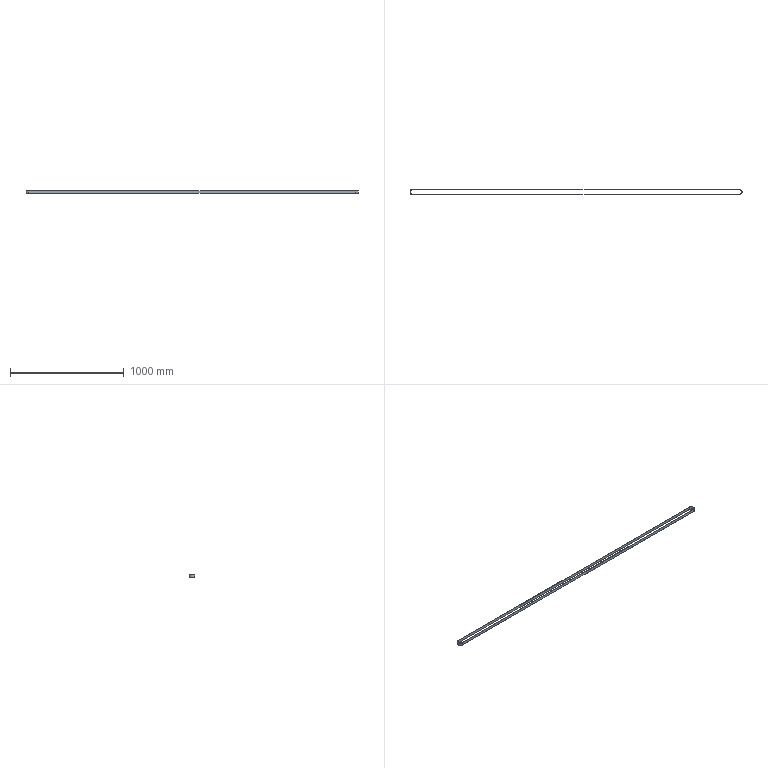Part | STEP file | Belt1-11^BPSP-03Fixture Return Conveyor Assembly_Default | 1 solid | 12 faces | box 2922 x 49 x 25 mm | volume 294683 mm3 | cylinder 6 | plane 6 | commonest cylinder face diameters 45 x3 49 x3
STEP:
#1=CARTESIAN_POINT('',(0.,0.,0.));
#2=DIRECTION('',(0.,0.,1.));
#3=DIRECTION('',(1.,0.,0.));
#4=AXIS2_PLACEMENT_3D('',#1,#2,#3);
#5=CARTESIAN_POINT('',(2873.,22.5,-25.));
#6=VERTEX_POINT('',#5);
#7=CARTESIAN_POINT('',(2873.,22.5,0.));
#8=VERTEX_POINT('',#7);
#9=CARTESIAN_POINT('',(2873.,22.5,-25.));
#10=DIRECTION('',(0.,0.,1.));
#11=VECTOR('',#10,1.);
#12=LINE('',#9,#11);
#13=CARTESIAN_POINT('',(2873.,0.000000009,-25.));
#14=DIRECTION('',(0.,0.,1.));
#15=DIRECTION('',(1.,0.,0.));
#16=AXIS2_PLACEMENT_3D('',#13,#14,#15);
#17=CYLINDRICAL_SURFACE('',#16,22.5);
#18=CARTESIAN_POINT('',(1.571,0.));
#19=DIRECTION('',(0.,1.));
#20=VECTOR('',#19,1.);
#21=LINE('',#18,#20);
#22=(GEOMETRIC_REPRESENTATION_CONTEXT(2)PARAMETRIC_REPRESENTATION_CONTEXT()REPRESENTATION_CONTEXT('',''));
#23=DEFINITIONAL_REPRESENTATION('',(#21),#22);
#24=PCURVE('',#17,#23);
#25=CARTESIAN_POINT('',(0.,22.5,-25.));
#26=DIRECTION('',(0.,1.,0.));
#27=DIRECTION('',(-1.,0.,0.));
#28=AXIS2_PLACEMENT_3D('',#25,#26,#27);
#29=PLANE('',#28);
#30=CARTESIAN_POINT('',(-2873.,0.));
#31=DIRECTION('',(0.,1.));
#32=VECTOR('',#31,1.);
#33=LINE('',#30,#32);
#34=(GEOMETRIC_REPRESENTATION_CONTEXT(2)PARAMETRIC_REPRESENTATION_CONTEXT()REPRESENTATION_CONTEXT('',''));
#35=DEFINITIONAL_REPRESENTATION('',(#33),#34);
#36=PCURVE('',#29,#35);
#37=SURFACE_CURVE('',#12,(#24,#36),.PCURVE_S1.);
#38=EDGE_CURVE('',#6,#8,#37,.T.);
#39=ORIENTED_EDGE('',*,*,#38,.T.);
#40=CARTESIAN_POINT('',(2895.5,0.000000009,0.));
#41=VERTEX_POINT('',#40);
#42=CARTESIAN_POINT('',(2873.,0.000000009,0.));
#43=DIRECTION('',(0.,0.,1.));
#44=DIRECTION('',(-1.,0.,0.));
#45=AXIS2_PLACEMENT_3D('',#42,#43,#44);
#46=CIRCLE('',#45,22.5);
#47=CARTESIAN_POINT('',(-3.142,25.));
#48=DIRECTION('',(1.,0.));
#49=VECTOR('',#48,1.);
#50=LINE('',#47,#49);
#51=(GEOMETRIC_REPRESENTATION_CONTEXT(2)PARAMETRIC_REPRESENTATION_CONTEXT()REPRESENTATION_CONTEXT('',''));
#52=DEFINITIONAL_REPRESENTATION('',(#50),#51);
#53=PCURVE('',#17,#52);
#54=CARTESIAN_POINT('',(0.,0.,0.));
#55=DIRECTION('',(0.,0.,-1.));
#56=DIRECTION('',(-1.,0.,0.));
#57=AXIS2_PLACEMENT_3D('',#54,#55,#56);
#58=PLANE('',#57);
#59=CARTESIAN_POINT('',(-2850.5,0.000000009));
#60=CARTESIAN_POINT('',(-2850.5,-38.971));
#61=CARTESIAN_POINT('',(-2884.25,-19.486));
#62=CARTESIAN_POINT('',(-2918.,0.000000009));
#63=CARTESIAN_POINT('',(-2884.25,19.486));
#64=CARTESIAN_POINT('',(-2850.5,38.971));
#65=CARTESIAN_POINT('',(-2850.5,0.000000009));
#66=(BOUNDED_CURVE()B_SPLINE_CURVE(2,(#59,#60,#61,#62,#63,#64,#65),.UNSPECIFIED.,.T.,.F.)B_SPLINE_CURVE_WITH_KNOTS((1,2,2,2,2,1),(-2.094,0.,2.094,4.189,6.283,8.378),.UNSPECIFIED.)CURVE()GEOMETRIC_REPRESENTATION_ITEM()RATIONAL_B_SPLINE_CURVE((1.,0.5,1.,0.5,1.,0.5,1.))REPRESENTATION_ITEM(''));
#67=(GEOMETRIC_REPRESENTATION_CONTEXT(2)PARAMETRIC_REPRESENTATION_CONTEXT()REPRESENTATION_CONTEXT('',''));
#68=DEFINITIONAL_REPRESENTATION('',(#66),#67);
#69=PCURVE('',#58,#68);
#70=SURFACE_CURVE('',#46,(#53,#69),.PCURVE_S1.);
#71=EDGE_CURVE('',#41,#8,#70,.T.);
#72=ORIENTED_EDGE('',*,*,#71,.F.);
#73=CARTESIAN_POINT('',(2895.5,0.000000009,-25.));
#74=VERTEX_POINT('',#73);
#75=CARTESIAN_POINT('',(2895.5,0.000000009,-25.));
#76=DIRECTION('',(0.,0.,1.));
#77=VECTOR('',#76,1.);
#78=LINE('',#75,#77);
#79=CARTESIAN_POINT('',(0.,0.));
#80=DIRECTION('',(0.,1.));
#81=VECTOR('',#80,1.);
#82=LINE('',#79,#81);
#83=(GEOMETRIC_REPRESENTATION_CONTEXT(2)PARAMETRIC_REPRESENTATION_CONTEXT()REPRESENTATION_CONTEXT('',''));
#84=DEFINITIONAL_REPRESENTATION('',(#82),#83);
#85=PCURVE('',#17,#84);
#86=CARTESIAN_POINT('',(2873.,0.000000009,-25.));
#87=DIRECTION('',(0.,0.,1.));
#88=DIRECTION('',(1.,0.,0.));
#89=AXIS2_PLACEMENT_3D('',#86,#87,#88);
#90=CYLINDRICAL_SURFACE('',#89,22.5);
#91=CARTESIAN_POINT('',(6.283,0.));
#92=DIRECTION('',(0.,1.));
#93=VECTOR('',#92,1.);
#94=LINE('',#91,#93);
#95=(GEOMETRIC_REPRESENTATION_CONTEXT(2)PARAMETRIC_REPRESENTATION_CONTEXT()REPRESENTATION_CONTEXT('',''));
#96=DEFINITIONAL_REPRESENTATION('',(#94),#95);
#97=PCURVE('',#90,#96);
#98=SURFACE_CURVE('',#78,(#85,#97),.PCURVE_S1.);
#99=EDGE_CURVE('',#74,#41,#98,.T.);
#100=ORIENTED_EDGE('',*,*,#99,.F.);
#101=CARTESIAN_POINT('',(2873.,0.000000009,-25.));
#102=DIRECTION('',(0.,0.,1.));
#103=DIRECTION('',(-1.,0.,0.));
#104=AXIS2_PLACEMENT_3D('',#101,#102,#103);
#105=CIRCLE('',#104,22.5);
#106=CARTESIAN_POINT('',(-3.142,0.));
#107=DIRECTION('',(1.,0.));
#108=VECTOR('',#107,1.);
#109=LINE('',#106,#108);
#110=(GEOMETRIC_REPRESENTATION_CONTEXT(2)PARAMETRIC_REPRESENTATION_CONTEXT()REPRESENTATION_CONTEXT('',''));
#111=DEFINITIONAL_REPRESENTATION('',(#109),#110);
#112=PCURVE('',#17,#111);
#113=CARTESIAN_POINT('',(0.,0.,-25.));
#114=DIRECTION('',(0.,0.,-1.));
#115=DIRECTION('',(-1.,0.,0.));
#116=AXIS2_PLACEMENT_3D('',#113,#114,#115);
#117=PLANE('',#116);
#118=CARTESIAN_POINT('',(-2850.5,0.000000009));
#119=CARTESIAN_POINT('',(-2850.5,-38.971));
#120=CARTESIAN_POINT('',(-2884.25,-19.486));
#121=CARTESIAN_POINT('',(-2918.,0.000000009));
#122=CARTESIAN_POINT('',(-2884.25,19.486));
#123=CARTESIAN_POINT('',(-2850.5,38.971));
#124=CARTESIAN_POINT('',(-2850.5,0.000000009));
#125=(BOUNDED_CURVE()B_SPLINE_CURVE(2,(#118,#119,#120,#121,#122,#123,#124),.UNSPECIFIED.,.T.,.F.)B_SPLINE_CURVE_WITH_KNOTS((1,2,2,2,2,1),(-2.094,0.,2.094,4.189,6.283,8.378),.UNSPECIFIED.)CURVE()GEOMETRIC_REPRESENTATION_ITEM()RATIONAL_B_SPLINE_CURVE((1.,0.5,1.,0.5,1.,0.5,1.))REPRESENTATION_ITEM(''));
#126=(GEOMETRIC_REPRESENTATION_CONTEXT(2)PARAMETRIC_REPRESENTATION_CONTEXT()REPRESENTATION_CONTEXT('',''));
#127=DEFINITIONAL_REPRESENTATION('',(#125),#126);
#128=PCURVE('',#117,#127);
#129=SURFACE_CURVE('',#105,(#112,#128),.PCURVE_S1.);
#130=EDGE_CURVE('',#74,#6,#129,.T.);
#131=ORIENTED_EDGE('',*,*,#130,.T.);
#132=EDGE_LOOP('',(#39,#72,#100,#131));
#133=FACE_BOUND('',#132,.F.);
#134=ADVANCED_FACE('',(#133),#17,.F.);
#135=CARTESIAN_POINT('',(2873.,-24.5,-25.));
#136=VERTEX_POINT('',#135);
#137=CARTESIAN_POINT('',(2897.5,0.000000009,-25.));
#138=VERTEX_POINT('',#137);
#139=CARTESIAN_POINT('',(2873.,0.000000009,-25.));
#140=DIRECTION('',(0.,0.,1.));
#141=DIRECTION('',(-1.,0.,0.));
#142=AXIS2_PLACEMENT_3D('',#139,#140,#141);
#143=CIRCLE('',#142,24.5);
#144=CARTESIAN_POINT('',(2873.,0.000000009,-25.));
#145=DIRECTION('',(0.,0.,1.));
#146=DIRECTION('',(1.,0.,0.));
#147=AXIS2_PLACEMENT_3D('',#144,#145,#146);
#148=CYLINDRICAL_SURFACE('',#147,24.5);
#149=CARTESIAN_POINT('',(3.142,0.));
#150=DIRECTION('',(1.,0.));
#151=VECTOR('',#150,1.);
#152=LINE('',#149,#151);
#153=(GEOMETRIC_REPRESENTATION_CONTEXT(2)PARAMETRIC_REPRESENTATION_CONTEXT()REPRESENTATION_CONTEXT('',''));
#154=DEFINITIONAL_REPRESENTATION('',(#152),#153);
#155=PCURVE('',#148,#154);
#156=CARTESIAN_POINT('',(-2848.5,0.000000009));
#157=CARTESIAN_POINT('',(-2848.5,-42.435));
#158=CARTESIAN_POINT('',(-2885.25,-21.218));
#159=CARTESIAN_POINT('',(-2922.,0.000000009));
#160=CARTESIAN_POINT('',(-2885.25,21.218));
#161=CARTESIAN_POINT('',(-2848.5,42.435));
#162=CARTESIAN_POINT('',(-2848.5,0.000000009));
#163=(BOUNDED_CURVE()B_SPLINE_CURVE(2,(#156,#157,#158,#159,#160,#161,#162),.UNSPECIFIED.,.T.,.F.)B_SPLINE_CURVE_WITH_KNOTS((1,2,2,2,2,1),(-2.094,0.,2.094,4.189,6.283,8.378),.UNSPECIFIED.)CURVE()GEOMETRIC_REPRESENTATION_ITEM()RATIONAL_B_SPLINE_CURVE((1.,0.5,1.,0.5,1.,0.5,1.))REPRESENTATION_ITEM(''));
#164=(GEOMETRIC_REPRESENTATION_CONTEXT(2)PARAMETRIC_REPRESENTATION_CONTEXT()REPRESENTATION_CONTEXT('',''));
#165=DEFINITIONAL_REPRESENTATION('',(#163),#164);
#166=PCURVE('',#117,#165);
#167=SURFACE_CURVE('',#143,(#155,#166),.PCURVE_S1.);
#168=EDGE_CURVE('',#136,#138,#167,.T.);
#169=ORIENTED_EDGE('',*,*,#168,.T.);
#170=CARTESIAN_POINT('',(2897.5,0.000000009,0.));
#171=VERTEX_POINT('',#170);
#172=CARTESIAN_POINT('',(2897.5,0.000000009,-25.));
#173=DIRECTION('',(0.,0.,1.));
#174=VECTOR('',#173,1.);
#175=LINE('',#172,#174);
#176=CARTESIAN_POINT('',(6.283,0.));
#177=DIRECTION('',(0.,1.));
#178=VECTOR('',#177,1.);
#179=LINE('',#176,#178);
#180=(GEOMETRIC_REPRESENTATION_CONTEXT(2)PARAMETRIC_REPRESENTATION_CONTEXT()REPRESENTATION_CONTEXT('',''));
#181=DEFINITIONAL_REPRESENTATION('',(#179),#180);
#182=PCURVE('',#148,#181);
#183=CARTESIAN_POINT('',(2873.,0.000000009,-25.));
#184=DIRECTION('',(0.,0.,1.));
#185=DIRECTION('',(1.,0.,0.));
#186=AXIS2_PLACEMENT_3D('',#183,#184,#185);
#187=CYLINDRICAL_SURFACE('',#186,24.5);
#188=CARTESIAN_POINT('',(0.,0.));
#189=DIRECTION('',(0.,1.));
#190=VECTOR('',#189,1.);
#191=LINE('',#188,#190);
#192=(GEOMETRIC_REPRESENTATION_CONTEXT(2)PARAMETRIC_REPRESENTATION_CONTEXT()REPRESENTATION_CONTEXT('',''));
#193=DEFINITIONAL_REPRESENTATION('',(#191),#192);
#194=PCURVE('',#187,#193);
#195=SURFACE_CURVE('',#175,(#182,#194),.PCURVE_S1.);
#196=EDGE_CURVE('',#138,#171,#195,.T.);
#197=ORIENTED_EDGE('',*,*,#196,.T.);
#198=CARTESIAN_POINT('',(2873.,-24.5,0.));
#199=VERTEX_POINT('',#198);
#200=CARTESIAN_POINT('',(2873.,0.000000009,0.));
#201=DIRECTION('',(0.,0.,1.));
#202=DIRECTION('',(-1.,0.,0.));
#203=AXIS2_PLACEMENT_3D('',#200,#201,#202);
#204=CIRCLE('',#203,24.5);
#205=CARTESIAN_POINT('',(3.142,25.));
#206=DIRECTION('',(1.,0.));
#207=VECTOR('',#206,1.);
#208=LINE('',#205,#207);
#209=(GEOMETRIC_REPRESENTATION_CONTEXT(2)PARAMETRIC_REPRESENTATION_CONTEXT()REPRESENTATION_CONTEXT('',''));
#210=DEFINITIONAL_REPRESENTATION('',(#208),#209);
#211=PCURVE('',#148,#210);
#212=CARTESIAN_POINT('',(-2848.5,0.000000009));
#213=CARTESIAN_POINT('',(-2848.5,-42.435));
#214=CARTESIAN_POINT('',(-2885.25,-21.218));
#215=CARTESIAN_POINT('',(-2922.,0.000000009));
#216=CARTESIAN_POINT('',(-2885.25,21.218));
#217=CARTESIAN_POINT('',(-2848.5,42.435));
#218=CARTESIAN_POINT('',(-2848.5,0.000000009));
#219=(BOUNDED_CURVE()B_SPLINE_CURVE(2,(#212,#213,#214,#215,#216,#217,#218),.UNSPECIFIED.,.T.,.F.)B_SPLINE_CURVE_WITH_KNOTS((1,2,2,2,2,1),(-2.094,0.,2.094,4.189,6.283,8.378),.UNSPECIFIED.)CURVE()GEOMETRIC_REPRESENTATION_ITEM()RATIONAL_B_SPLINE_CURVE((1.,0.5,1.,0.5,1.,0.5,1.))REPRESENTATION_ITEM(''));
#220=(GEOMETRIC_REPRESENTATION_CONTEXT(2)PARAMETRIC_REPRESENTATION_CONTEXT()REPRESENTATION_CONTEXT('',''));
#221=DEFINITIONAL_REPRESENTATION('',(#219),#220);
#222=PCURVE('',#58,#221);
#223=SURFACE_CURVE('',#204,(#211,#222),.PCURVE_S1.);
#224=EDGE_CURVE('',#199,#171,#223,.T.);
#225=ORIENTED_EDGE('',*,*,#224,.F.);
#226=CARTESIAN_POINT('',(2873.,-24.5,-25.));
#227=DIRECTION('',(0.,0.,1.));
#228=VECTOR('',#227,1.);
#229=LINE('',#226,#228);
#230=CARTESIAN_POINT('',(4.712,0.));
#231=DIRECTION('',(0.,1.));
#232=VECTOR('',#231,1.);
#233=LINE('',#230,#232);
#234=(GEOMETRIC_REPRESENTATION_CONTEXT(2)PARAMETRIC_REPRESENTATION_CONTEXT()REPRESENTATION_CONTEXT('',''));
#235=DEFINITIONAL_REPRESENTATION('',(#233),#234);
#236=PCURVE('',#148,#235);
#237=CARTESIAN_POINT('',(2873.,-24.5,-25.));
#238=DIRECTION('',(0.,-1.,0.));
#239=DIRECTION('',(1.,0.,0.));
#240=AXIS2_PLACEMENT_3D('',#237,#238,#239);
#241=PLANE('',#240);
#242=CARTESIAN_POINT('',(0.,0.));
#243=DIRECTION('',(0.,1.));
#244=VECTOR('',#243,1.);
#245=LINE('',#242,#244);
#246=(GEOMETRIC_REPRESENTATION_CONTEXT(2)PARAMETRIC_REPRESENTATION_CONTEXT()REPRESENTATION_CONTEXT('',''));
#247=DEFINITIONAL_REPRESENTATION('',(#245),#246);
#248=PCURVE('',#241,#247);
#249=SURFACE_CURVE('',#229,(#236,#248),.PCURVE_S1.);
#250=EDGE_CURVE('',#136,#199,#249,.T.);
#251=ORIENTED_EDGE('',*,*,#250,.F.);
#252=EDGE_LOOP('',(#169,#197,#225,#251));
#253=FACE_BOUND('',#252,.T.);
#254=ADVANCED_FACE('',(#253),#148,.T.);
#255=CARTESIAN_POINT('',(0.,24.5,-25.));
#256=VERTEX_POINT('',#255);
#257=CARTESIAN_POINT('',(0.,-24.5,-25.));
#258=VERTEX_POINT('',#257);
#259=CARTESIAN_POINT('',(0.,0.,-25.));
#260=DIRECTION('',(0.,0.,1.));
#261=DIRECTION('',(-1.,0.,0.));
#262=AXIS2_PLACEMENT_3D('',#259,#260,#261);
#263=CIRCLE('',#262,24.5);
#264=CARTESIAN_POINT('',(24.5,0.));
#265=CARTESIAN_POINT('',(24.5,-42.435));
#266=CARTESIAN_POINT('',(-12.25,-21.218));
#267=CARTESIAN_POINT('',(-49.,0.));
#268=CARTESIAN_POINT('',(-12.25,21.218));
#269=CARTESIAN_POINT('',(24.5,42.435));
#270=CARTESIAN_POINT('',(24.5,0.));
#271=(BOUNDED_CURVE()B_SPLINE_CURVE(2,(#264,#265,#266,#267,#268,#269,#270),.UNSPECIFIED.,.T.,.F.)B_SPLINE_CURVE_WITH_KNOTS((1,2,2,2,2,1),(-2.094,0.,2.094,4.189,6.283,8.378),.UNSPECIFIED.)CURVE()GEOMETRIC_REPRESENTATION_ITEM()RATIONAL_B_SPLINE_CURVE((1.,0.5,1.,0.5,1.,0.5,1.))REPRESENTATION_ITEM(''));
#272=(GEOMETRIC_REPRESENTATION_CONTEXT(2)PARAMETRIC_REPRESENTATION_CONTEXT()REPRESENTATION_CONTEXT('',''));
#273=DEFINITIONAL_REPRESENTATION('',(#271),#272);
#274=PCURVE('',#117,#273);
#275=CARTESIAN_POINT('',(0.,0.,-25.));
#276=DIRECTION('',(0.,0.,1.));
#277=DIRECTION('',(1.,0.,0.));
#278=AXIS2_PLACEMENT_3D('',#275,#276,#277);
#279=CYLINDRICAL_SURFACE('',#278,24.5);
#280=CARTESIAN_POINT('',(-3.142,0.));
#281=DIRECTION('',(1.,0.));
#282=VECTOR('',#281,1.);
#283=LINE('',#280,#282);
#284=(GEOMETRIC_REPRESENTATION_CONTEXT(2)PARAMETRIC_REPRESENTATION_CONTEXT()REPRESENTATION_CONTEXT('',''));
#285=DEFINITIONAL_REPRESENTATION('',(#283),#284);
#286=PCURVE('',#279,#285);
#287=SURFACE_CURVE('',#263,(#274,#286),.PCURVE_S1.);
#288=EDGE_CURVE('',#256,#258,#287,.T.);
#289=ORIENTED_EDGE('',*,*,#288,.F.);
#290=CARTESIAN_POINT('',(2873.,24.5,-25.));
#291=VERTEX_POINT('',#290);
#292=CARTESIAN_POINT('',(0.,24.5,-25.));
#293=DIRECTION('',(-1.,0.,0.));
#294=VECTOR('',#293,1.);
#295=LINE('',#292,#294);
#296=CARTESIAN_POINT('',(0.,24.5));
#297=DIRECTION('',(1.,0.));
#298=VECTOR('',#297,1.);
#299=LINE('',#296,#298);
#300=(GEOMETRIC_REPRESENTATION_CONTEXT(2)PARAMETRIC_REPRESENTATION_CONTEXT()REPRESENTATION_CONTEXT('',''));
#301=DEFINITIONAL_REPRESENTATION('',(#299),#300);
#302=PCURVE('',#117,#301);
#303=CARTESIAN_POINT('',(0.,24.5,-25.));
#304=DIRECTION('',(0.,1.,0.));
#305=DIRECTION('',(-1.,0.,0.));
#306=AXIS2_PLACEMENT_3D('',#303,#304,#305);
#307=PLANE('',#306);
#308=CARTESIAN_POINT('',(0.,0.));
#309=DIRECTION('',(1.,0.));
#310=VECTOR('',#309,1.);
#311=LINE('',#308,#310);
#312=(GEOMETRIC_REPRESENTATION_CONTEXT(2)PARAMETRIC_REPRESENTATION_CONTEXT()REPRESENTATION_CONTEXT('',''));
#313=DEFINITIONAL_REPRESENTATION('',(#311),#312);
#314=PCURVE('',#307,#313);
#315=SURFACE_CURVE('',#295,(#302,#314),.PCURVE_S1.);
#316=EDGE_CURVE('',#291,#256,#315,.T.);
#317=ORIENTED_EDGE('',*,*,#316,.F.);
#318=CARTESIAN_POINT('',(2873.,0.000000009,-25.));
#319=DIRECTION('',(0.,0.,1.));
#320=DIRECTION('',(-1.,0.,0.));
#321=AXIS2_PLACEMENT_3D('',#318,#319,#320);
#322=CIRCLE('',#321,24.5);
#323=CARTESIAN_POINT('',(-2848.5,0.000000009));
#324=CARTESIAN_POINT('',(-2848.5,-42.435));
#325=CARTESIAN_POINT('',(-2885.25,-21.218));
#326=CARTESIAN_POINT('',(-2922.,0.000000009));
#327=CARTESIAN_POINT('',(-2885.25,21.218));
#328=CARTESIAN_POINT('',(-2848.5,42.435));
#329=CARTESIAN_POINT('',(-2848.5,0.000000009));
#330=(BOUNDED_CURVE()B_SPLINE_CURVE(2,(#323,#324,#325,#326,#327,#328,#329),.UNSPECIFIED.,.T.,.F.)B_SPLINE_CURVE_WITH_KNOTS((1,2,2,2,2,1),(-2.094,0.,2.094,4.189,6.283,8.378),.UNSPECIFIED.)CURVE()GEOMETRIC_REPRESENTATION_ITEM()RATIONAL_B_SPLINE_CURVE((1.,0.5,1.,0.5,1.,0.5,1.))REPRESENTATION_ITEM(''));
#331=(GEOMETRIC_REPRESENTATION_CONTEXT(2)PARAMETRIC_REPRESENTATION_CONTEXT()REPRESENTATION_CONTEXT('',''));
#332=DEFINITIONAL_REPRESENTATION('',(#330),#331);
#333=PCURVE('',#117,#332);
#334=CARTESIAN_POINT('',(-3.142,0.));
#335=DIRECTION('',(1.,0.));
#336=VECTOR('',#335,1.);
#337=LINE('',#334,#336);
#338=(GEOMETRIC_REPRESENTATION_CONTEXT(2)PARAMETRIC_REPRESENTATION_CONTEXT()REPRESENTATION_CONTEXT('',''));
#339=DEFINITIONAL_REPRESENTATION('',(#337),#338);
#340=PCURVE('',#187,#339);
#341=SURFACE_CURVE('',#322,(#333,#340),.PCURVE_S1.);
#342=EDGE_CURVE('',#138,#291,#341,.T.);
#343=ORIENTED_EDGE('',*,*,#342,.F.);
#344=ORIENTED_EDGE('',*,*,#168,.F.);
#345=CARTESIAN_POINT('',(2873.,-24.5,-25.));
#346=DIRECTION('',(1.,0.,0.));
#347=VECTOR('',#346,1.);
#348=LINE('',#345,#347);
#349=CARTESIAN_POINT('',(-2873.,-24.5));
#350=DIRECTION('',(-1.,0.));
#351=VECTOR('',#350,1.);
#352=LINE('',#349,#351);
#353=(GEOMETRIC_REPRESENTATION_CONTEXT(2)PARAMETRIC_REPRESENTATION_CONTEXT()REPRESENTATION_CONTEXT('',''));
#354=DEFINITIONAL_REPRESENTATION('',(#352),#353);
#355=PCURVE('',#117,#354);
#356=CARTESIAN_POINT('',(0.,0.));
#357=DIRECTION('',(1.,0.));
#358=VECTOR('',#357,1.);
#359=LINE('',#356,#358);
#360=(GEOMETRIC_REPRESENTATION_CONTEXT(2)PARAMETRIC_REPRESENTATION_CONTEXT()REPRESENTATION_CONTEXT('',''));
#361=DEFINITIONAL_REPRESENTATION('',(#359),#360);
#362=PCURVE('',#241,#361);
#363=SURFACE_CURVE('',#348,(#355,#362),.PCURVE_S1.);
#364=EDGE_CURVE('',#258,#136,#363,.T.);
#365=ORIENTED_EDGE('',*,*,#364,.F.);
#366=EDGE_LOOP('',(#289,#317,#343,#344,#365));
#367=FACE_BOUND('',#366,.T.);
#368=CARTESIAN_POINT('',(0.,22.5,-25.));
#369=VERTEX_POINT('',#368);
#370=CARTESIAN_POINT('',(0.,22.5,-25.));
#371=DIRECTION('',(-1.,0.,0.));
#372=VECTOR('',#371,1.);
#373=LINE('',#370,#372);
#374=CARTESIAN_POINT('',(0.,22.5));
#375=DIRECTION('',(1.,0.));
#376=VECTOR('',#375,1.);
#377=LINE('',#374,#376);
#378=(GEOMETRIC_REPRESENTATION_CONTEXT(2)PARAMETRIC_REPRESENTATION_CONTEXT()REPRESENTATION_CONTEXT('',''));
#379=DEFINITIONAL_REPRESENTATION('',(#377),#378);
#380=PCURVE('',#117,#379);
#381=CARTESIAN_POINT('',(0.,0.));
#382=DIRECTION('',(1.,0.));
#383=VECTOR('',#382,1.);
#384=LINE('',#381,#383);
#385=(GEOMETRIC_REPRESENTATION_CONTEXT(2)PARAMETRIC_REPRESENTATION_CONTEXT()REPRESENTATION_CONTEXT('',''));
#386=DEFINITIONAL_REPRESENTATION('',(#384),#385);
#387=PCURVE('',#29,#386);
#388=SURFACE_CURVE('',#373,(#380,#387),.PCURVE_S1.);
#389=EDGE_CURVE('',#6,#369,#388,.T.);
#390=ORIENTED_EDGE('',*,*,#389,.T.);
#391=CARTESIAN_POINT('',(0.,-22.5,-25.));
#392=VERTEX_POINT('',#391);
#393=CARTESIAN_POINT('',(0.,0.,-25.));
#394=DIRECTION('',(0.,0.,1.));
#395=DIRECTION('',(-1.,0.,0.));
#396=AXIS2_PLACEMENT_3D('',#393,#394,#395);
#397=CIRCLE('',#396,22.5);
#398=CARTESIAN_POINT('',(22.5,0.));
#399=CARTESIAN_POINT('',(22.5,-38.971));
#400=CARTESIAN_POINT('',(-11.25,-19.486));
#401=CARTESIAN_POINT('',(-45.,0.));
#402=CARTESIAN_POINT('',(-11.25,19.486));
#403=CARTESIAN_POINT('',(22.5,38.971));
#404=CARTESIAN_POINT('',(22.5,0.));
#405=(BOUNDED_CURVE()B_SPLINE_CURVE(2,(#398,#399,#400,#401,#402,#403,#404),.UNSPECIFIED.,.T.,.F.)B_SPLINE_CURVE_WITH_KNOTS((1,2,2,2,2,1),(-2.094,0.,2.094,4.189,6.283,8.378),.UNSPECIFIED.)CURVE()GEOMETRIC_REPRESENTATION_ITEM()RATIONAL_B_SPLINE_CURVE((1.,0.5,1.,0.5,1.,0.5,1.))REPRESENTATION_ITEM(''));
#406=(GEOMETRIC_REPRESENTATION_CONTEXT(2)PARAMETRIC_REPRESENTATION_CONTEXT()REPRESENTATION_CONTEXT('',''));
#407=DEFINITIONAL_REPRESENTATION('',(#405),#406);
#408=PCURVE('',#117,#407);
#409=CARTESIAN_POINT('',(0.,0.,-25.));
#410=DIRECTION('',(0.,0.,1.));
#411=DIRECTION('',(1.,0.,0.));
#412=AXIS2_PLACEMENT_3D('',#409,#410,#411);
#413=CYLINDRICAL_SURFACE('',#412,22.5);
#414=CARTESIAN_POINT('',(-3.142,0.));
#415=DIRECTION('',(1.,0.));
#416=VECTOR('',#415,1.);
#417=LINE('',#414,#416);
#418=(GEOMETRIC_REPRESENTATION_CONTEXT(2)PARAMETRIC_REPRESENTATION_CONTEXT()REPRESENTATION_CONTEXT('',''));
#419=DEFINITIONAL_REPRESENTATION('',(#417),#418);
#420=PCURVE('',#413,#419);
#421=SURFACE_CURVE('',#397,(#408,#420),.PCURVE_S1.);
#422=EDGE_CURVE('',#369,#392,#421,.T.);
#423=ORIENTED_EDGE('',*,*,#422,.T.);
#424=CARTESIAN_POINT('',(2873.,-22.5,-25.));
#425=VERTEX_POINT('',#424);
#426=CARTESIAN_POINT('',(2873.,-22.5,-25.));
#427=DIRECTION('',(1.,0.,0.));
#428=VECTOR('',#427,1.);
#429=LINE('',#426,#428);
#430=CARTESIAN_POINT('',(-2873.,-22.5));
#431=DIRECTION('',(-1.,0.));
#432=VECTOR('',#431,1.);
#433=LINE('',#430,#432);
#434=(GEOMETRIC_REPRESENTATION_CONTEXT(2)PARAMETRIC_REPRESENTATION_CONTEXT()REPRESENTATION_CONTEXT('',''));
#435=DEFINITIONAL_REPRESENTATION('',(#433),#434);
#436=PCURVE('',#117,#435);
#437=CARTESIAN_POINT('',(2873.,-22.5,-25.));
#438=DIRECTION('',(0.,-1.,0.));
#439=DIRECTION('',(1.,0.,0.));
#440=AXIS2_PLACEMENT_3D('',#437,#438,#439);
#441=PLANE('',#440);
#442=CARTESIAN_POINT('',(0.,0.));
#443=DIRECTION('',(1.,0.));
#444=VECTOR('',#443,1.);
#445=LINE('',#442,#444);
#446=(GEOMETRIC_REPRESENTATION_CONTEXT(2)PARAMETRIC_REPRESENTATION_CONTEXT()REPRESENTATION_CONTEXT('',''));
#447=DEFINITIONAL_REPRESENTATION('',(#445),#446);
#448=PCURVE('',#441,#447);
#449=SURFACE_CURVE('',#429,(#436,#448),.PCURVE_S1.);
#450=EDGE_CURVE('',#392,#425,#449,.T.);
#451=ORIENTED_EDGE('',*,*,#450,.T.);
#452=CARTESIAN_POINT('',(2873.,0.000000009,-25.));
#453=DIRECTION('',(0.,0.,1.));
#454=DIRECTION('',(-1.,0.,0.));
#455=AXIS2_PLACEMENT_3D('',#452,#453,#454);
#456=CIRCLE('',#455,22.5);
#457=CARTESIAN_POINT('',(-2850.5,0.000000009));
#458=CARTESIAN_POINT('',(-2850.5,-38.971));
#459=CARTESIAN_POINT('',(-2884.25,-19.486));
#460=CARTESIAN_POINT('',(-2918.,0.000000009));
#461=CARTESIAN_POINT('',(-2884.25,19.486));
#462=CARTESIAN_POINT('',(-2850.5,38.971));
#463=CARTESIAN_POINT('',(-2850.5,0.000000009));
#464=(BOUNDED_CURVE()B_SPLINE_CURVE(2,(#457,#458,#459,#460,#461,#462,#463),.UNSPECIFIED.,.T.,.F.)B_SPLINE_CURVE_WITH_KNOTS((1,2,2,2,2,1),(-2.094,0.,2.094,4.189,6.283,8.378),.UNSPECIFIED.)CURVE()GEOMETRIC_REPRESENTATION_ITEM()RATIONAL_B_SPLINE_CURVE((1.,0.5,1.,0.5,1.,0.5,1.))REPRESENTATION_ITEM(''));
#465=(GEOMETRIC_REPRESENTATION_CONTEXT(2)PARAMETRIC_REPRESENTATION_CONTEXT()REPRESENTATION_CONTEXT('',''));
#466=DEFINITIONAL_REPRESENTATION('',(#464),#465);
#467=PCURVE('',#117,#466);
#468=CARTESIAN_POINT('',(3.142,0.));
#469=DIRECTION('',(1.,0.));
#470=VECTOR('',#469,1.);
#471=LINE('',#468,#470);
#472=(GEOMETRIC_REPRESENTATION_CONTEXT(2)PARAMETRIC_REPRESENTATION_CONTEXT()REPRESENTATION_CONTEXT('',''));
#473=DEFINITIONAL_REPRESENTATION('',(#471),#472);
#474=PCURVE('',#90,#473);
#475=SURFACE_CURVE('',#456,(#467,#474),.PCURVE_S1.);
#476=EDGE_CURVE('',#425,#74,#475,.T.);
#477=ORIENTED_EDGE('',*,*,#476,.T.);
#478=ORIENTED_EDGE('',*,*,#130,.T.);
#479=EDGE_LOOP('',(#390,#423,#451,#477,#478));
#480=FACE_BOUND('',#479,.T.);
#481=ADVANCED_FACE('',(#367,#480),#117,.T.);
#482=CARTESIAN_POINT('',(0.,24.5,0.));
#483=VERTEX_POINT('',#482);
#484=CARTESIAN_POINT('',(0.,-24.5,0.));
#485=VERTEX_POINT('',#484);
#486=CARTESIAN_POINT('',(0.,0.,0.));
#487=DIRECTION('',(0.,0.,1.));
#488=DIRECTION('',(-1.,0.,0.));
#489=AXIS2_PLACEMENT_3D('',#486,#487,#488);
#490=CIRCLE('',#489,24.5);
#491=CARTESIAN_POINT('',(24.5,0.));
#492=CARTESIAN_POINT('',(24.5,-42.435));
#493=CARTESIAN_POINT('',(-12.25,-21.218));
#494=CARTESIAN_POINT('',(-49.,0.));
#495=CARTESIAN_POINT('',(-12.25,21.218));
#496=CARTESIAN_POINT('',(24.5,42.435));
#497=CARTESIAN_POINT('',(24.5,0.));
#498=(BOUNDED_CURVE()B_SPLINE_CURVE(2,(#491,#492,#493,#494,#495,#496,#497),.UNSPECIFIED.,.T.,.F.)B_SPLINE_CURVE_WITH_KNOTS((1,2,2,2,2,1),(-2.094,0.,2.094,4.189,6.283,8.378),.UNSPECIFIED.)CURVE()GEOMETRIC_REPRESENTATION_ITEM()RATIONAL_B_SPLINE_CURVE((1.,0.5,1.,0.5,1.,0.5,1.))REPRESENTATION_ITEM(''));
#499=(GEOMETRIC_REPRESENTATION_CONTEXT(2)PARAMETRIC_REPRESENTATION_CONTEXT()REPRESENTATION_CONTEXT('',''));
#500=DEFINITIONAL_REPRESENTATION('',(#498),#499);
#501=PCURVE('',#58,#500);
#502=CARTESIAN_POINT('',(-3.142,25.));
#503=DIRECTION('',(1.,0.));
#504=VECTOR('',#503,1.);
#505=LINE('',#502,#504);
#506=(GEOMETRIC_REPRESENTATION_CONTEXT(2)PARAMETRIC_REPRESENTATION_CONTEXT()REPRESENTATION_CONTEXT('',''));
#507=DEFINITIONAL_REPRESENTATION('',(#505),#506);
#508=PCURVE('',#279,#507);
#509=SURFACE_CURVE('',#490,(#501,#508),.PCURVE_S1.);
#510=EDGE_CURVE('',#483,#485,#509,.T.);
#511=ORIENTED_EDGE('',*,*,#510,.T.);
#512=CARTESIAN_POINT('',(2873.,-24.5,0.));
#513=DIRECTION('',(1.,0.,0.));
#514=VECTOR('',#513,1.);
#515=LINE('',#512,#514);
#516=CARTESIAN_POINT('',(-2873.,-24.5));
#517=DIRECTION('',(-1.,0.));
#518=VECTOR('',#517,1.);
#519=LINE('',#516,#518);
#520=(GEOMETRIC_REPRESENTATION_CONTEXT(2)PARAMETRIC_REPRESENTATION_CONTEXT()REPRESENTATION_CONTEXT('',''));
#521=DEFINITIONAL_REPRESENTATION('',(#519),#520);
#522=PCURVE('',#58,#521);
#523=CARTESIAN_POINT('',(0.,25.));
#524=DIRECTION('',(1.,0.));
#525=VECTOR('',#524,1.);
#526=LINE('',#523,#525);
#527=(GEOMETRIC_REPRESENTATION_CONTEXT(2)PARAMETRIC_REPRESENTATION_CONTEXT()REPRESENTATION_CONTEXT('',''));
#528=DEFINITIONAL_REPRESENTATION('',(#526),#527);
#529=PCURVE('',#241,#528);
#530=SURFACE_CURVE('',#515,(#522,#529),.PCURVE_S1.);
#531=EDGE_CURVE('',#485,#199,#530,.T.);
#532=ORIENTED_EDGE('',*,*,#531,.T.);
#533=ORIENTED_EDGE('',*,*,#224,.T.);
#534=CARTESIAN_POINT('',(2873.,24.5,0.));
#535=VERTEX_POINT('',#534);
#536=CARTESIAN_POINT('',(2873.,0.000000009,0.));
#537=DIRECTION('',(0.,0.,1.));
#538=DIRECTION('',(-1.,0.,0.));
#539=AXIS2_PLACEMENT_3D('',#536,#537,#538);
#540=CIRCLE('',#539,24.5);
#541=CARTESIAN_POINT('',(-2848.5,0.000000009));
#542=CARTESIAN_POINT('',(-2848.5,-42.435));
#543=CARTESIAN_POINT('',(-2885.25,-21.218));
#544=CARTESIAN_POINT('',(-2922.,0.000000009));
#545=CARTESIAN_POINT('',(-2885.25,21.218));
#546=CARTESIAN_POINT('',(-2848.5,42.435));
#547=CARTESIAN_POINT('',(-2848.5,0.000000009));
#548=(BOUNDED_CURVE()B_SPLINE_CURVE(2,(#541,#542,#543,#544,#545,#546,#547),.UNSPECIFIED.,.T.,.F.)B_SPLINE_CURVE_WITH_KNOTS((1,2,2,2,2,1),(-2.094,0.,2.094,4.189,6.283,8.378),.UNSPECIFIED.)CURVE()GEOMETRIC_REPRESENTATION_ITEM()RATIONAL_B_SPLINE_CURVE((1.,0.5,1.,0.5,1.,0.5,1.))REPRESENTATION_ITEM(''));
#549=(GEOMETRIC_REPRESENTATION_CONTEXT(2)PARAMETRIC_REPRESENTATION_CONTEXT()REPRESENTATION_CONTEXT('',''));
#550=DEFINITIONAL_REPRESENTATION('',(#548),#549);
#551=PCURVE('',#58,#550);
#552=CARTESIAN_POINT('',(-3.142,25.));
#553=DIRECTION('',(1.,0.));
#554=VECTOR('',#553,1.);
#555=LINE('',#552,#554);
#556=(GEOMETRIC_REPRESENTATION_CONTEXT(2)PARAMETRIC_REPRESENTATION_CONTEXT()REPRESENTATION_CONTEXT('',''));
#557=DEFINITIONAL_REPRESENTATION('',(#555),#556);
#558=PCURVE('',#187,#557);
#559=SURFACE_CURVE('',#540,(#551,#558),.PCURVE_S1.);
#560=EDGE_CURVE('',#171,#535,#559,.T.);
#561=ORIENTED_EDGE('',*,*,#560,.T.);
#562=CARTESIAN_POINT('',(0.,24.5,0.));
#563=DIRECTION('',(-1.,0.,0.));
#564=VECTOR('',#563,1.);
#565=LINE('',#562,#564);
#566=CARTESIAN_POINT('',(0.,24.5));
#567=DIRECTION('',(1.,0.));
#568=VECTOR('',#567,1.);
#569=LINE('',#566,#568);
#570=(GEOMETRIC_REPRESENTATION_CONTEXT(2)PARAMETRIC_REPRESENTATION_CONTEXT()REPRESENTATION_CONTEXT('',''));
#571=DEFINITIONAL_REPRESENTATION('',(#569),#570);
#572=PCURVE('',#58,#571);
#573=CARTESIAN_POINT('',(0.,25.));
#574=DIRECTION('',(1.,0.));
#575=VECTOR('',#574,1.);
#576=LINE('',#573,#575);
#577=(GEOMETRIC_REPRESENTATION_CONTEXT(2)PARAMETRIC_REPRESENTATION_CONTEXT()REPRESENTATION_CONTEXT('',''));
#578=DEFINITIONAL_REPRESENTATION('',(#576),#577);
#579=PCURVE('',#307,#578);
#580=SURFACE_CURVE('',#565,(#572,#579),.PCURVE_S1.);
#581=EDGE_CURVE('',#535,#483,#580,.T.);
#582=ORIENTED_EDGE('',*,*,#581,.T.);
#583=EDGE_LOOP('',(#511,#532,#533,#561,#582));
#584=FACE_BOUND('',#583,.T.);
#585=CARTESIAN_POINT('',(0.,22.5,0.));
#586=VERTEX_POINT('',#585);
#587=CARTESIAN_POINT('',(0.,-22.5,0.));
#588=VERTEX_POINT('',#587);
#589=CARTESIAN_POINT('',(0.,0.,0.));
#590=DIRECTION('',(0.,0.,1.));
#591=DIRECTION('',(-1.,0.,0.));
#592=AXIS2_PLACEMENT_3D('',#589,#590,#591);
#593=CIRCLE('',#592,22.5);
#594=CARTESIAN_POINT('',(22.5,0.));
#595=CARTESIAN_POINT('',(22.5,-38.971));
#596=CARTESIAN_POINT('',(-11.25,-19.486));
#597=CARTESIAN_POINT('',(-45.,0.));
#598=CARTESIAN_POINT('',(-11.25,19.486));
#599=CARTESIAN_POINT('',(22.5,38.971));
#600=CARTESIAN_POINT('',(22.5,0.));
#601=(BOUNDED_CURVE()B_SPLINE_CURVE(2,(#594,#595,#596,#597,#598,#599,#600),.UNSPECIFIED.,.T.,.F.)B_SPLINE_CURVE_WITH_KNOTS((1,2,2,2,2,1),(-2.094,0.,2.094,4.189,6.283,8.378),.UNSPECIFIED.)CURVE()GEOMETRIC_REPRESENTATION_ITEM()RATIONAL_B_SPLINE_CURVE((1.,0.5,1.,0.5,1.,0.5,1.))REPRESENTATION_ITEM(''));
#602=(GEOMETRIC_REPRESENTATION_CONTEXT(2)PARAMETRIC_REPRESENTATION_CONTEXT()REPRESENTATION_CONTEXT('',''));
#603=DEFINITIONAL_REPRESENTATION('',(#601),#602);
#604=PCURVE('',#58,#603);
#605=CARTESIAN_POINT('',(-3.142,25.));
#606=DIRECTION('',(1.,0.));
#607=VECTOR('',#606,1.);
#608=LINE('',#605,#607);
#609=(GEOMETRIC_REPRESENTATION_CONTEXT(2)PARAMETRIC_REPRESENTATION_CONTEXT()REPRESENTATION_CONTEXT('',''));
#610=DEFINITIONAL_REPRESENTATION('',(#608),#609);
#611=PCURVE('',#413,#610);
#612=SURFACE_CURVE('',#593,(#604,#611),.PCURVE_S1.);
#613=EDGE_CURVE('',#586,#588,#612,.T.);
#614=ORIENTED_EDGE('',*,*,#613,.F.);
#615=CARTESIAN_POINT('',(0.,22.5,0.));
#616=DIRECTION('',(-1.,0.,0.));
#617=VECTOR('',#616,1.);
#618=LINE('',#615,#617);
#619=CARTESIAN_POINT('',(0.,22.5));
#620=DIRECTION('',(1.,0.));
#621=VECTOR('',#620,1.);
#622=LINE('',#619,#621);
#623=(GEOMETRIC_REPRESENTATION_CONTEXT(2)PARAMETRIC_REPRESENTATION_CONTEXT()REPRESENTATION_CONTEXT('',''));
#624=DEFINITIONAL_REPRESENTATION('',(#622),#623);
#625=PCURVE('',#58,#624);
#626=CARTESIAN_POINT('',(0.,25.));
#627=DIRECTION('',(1.,0.));
#628=VECTOR('',#627,1.);
#629=LINE('',#626,#628);
#630=(GEOMETRIC_REPRESENTATION_CONTEXT(2)PARAMETRIC_REPRESENTATION_CONTEXT()REPRESENTATION_CONTEXT('',''));
#631=DEFINITIONAL_REPRESENTATION('',(#629),#630);
#632=PCURVE('',#29,#631);
#633=SURFACE_CURVE('',#618,(#625,#632),.PCURVE_S1.);
#634=EDGE_CURVE('',#8,#586,#633,.T.);
#635=ORIENTED_EDGE('',*,*,#634,.F.);
#636=ORIENTED_EDGE('',*,*,#71,.F.);
#637=CARTESIAN_POINT('',(2873.,-22.5,0.));
#638=VERTEX_POINT('',#637);
#639=CARTESIAN_POINT('',(2873.,0.000000009,0.));
#640=DIRECTION('',(0.,0.,1.));
#641=DIRECTION('',(-1.,0.,0.));
#642=AXIS2_PLACEMENT_3D('',#639,#640,#641);
#643=CIRCLE('',#642,22.5);
#644=CARTESIAN_POINT('',(-2850.5,0.000000009));
#645=CARTESIAN_POINT('',(-2850.5,-38.971));
#646=CARTESIAN_POINT('',(-2884.25,-19.486));
#647=CARTESIAN_POINT('',(-2918.,0.000000009));
#648=CARTESIAN_POINT('',(-2884.25,19.486));
#649=CARTESIAN_POINT('',(-2850.5,38.971));
#650=CARTESIAN_POINT('',(-2850.5,0.000000009));
#651=(BOUNDED_CURVE()B_SPLINE_CURVE(2,(#644,#645,#646,#647,#648,#649,#650),.UNSPECIFIED.,.T.,.F.)B_SPLINE_CURVE_WITH_KNOTS((1,2,2,2,2,1),(-2.094,0.,2.094,4.189,6.283,8.378),.UNSPECIFIED.)CURVE()GEOMETRIC_REPRESENTATION_ITEM()RATIONAL_B_SPLINE_CURVE((1.,0.5,1.,0.5,1.,0.5,1.))REPRESENTATION_ITEM(''));
#652=(GEOMETRIC_REPRESENTATION_CONTEXT(2)PARAMETRIC_REPRESENTATION_CONTEXT()REPRESENTATION_CONTEXT('',''));
#653=DEFINITIONAL_REPRESENTATION('',(#651),#652);
#654=PCURVE('',#58,#653);
#655=CARTESIAN_POINT('',(3.142,25.));
#656=DIRECTION('',(1.,0.));
#657=VECTOR('',#656,1.);
#658=LINE('',#655,#657);
#659=(GEOMETRIC_REPRESENTATION_CONTEXT(2)PARAMETRIC_REPRESENTATION_CONTEXT()REPRESENTATION_CONTEXT('',''));
#660=DEFINITIONAL_REPRESENTATION('',(#658),#659);
#661=PCURVE('',#90,#660);
#662=SURFACE_CURVE('',#643,(#654,#661),.PCURVE_S1.);
#663=EDGE_CURVE('',#638,#41,#662,.T.);
#664=ORIENTED_EDGE('',*,*,#663,.F.);
#665=CARTESIAN_POINT('',(2873.,-22.5,0.));
#666=DIRECTION('',(1.,0.,0.));
#667=VECTOR('',#666,1.);
#668=LINE('',#665,#667);
#669=CARTESIAN_POINT('',(-2873.,-22.5));
#670=DIRECTION('',(-1.,0.));
#671=VECTOR('',#670,1.);
#672=LINE('',#669,#671);
#673=(GEOMETRIC_REPRESENTATION_CONTEXT(2)PARAMETRIC_REPRESENTATION_CONTEXT()REPRESENTATION_CONTEXT('',''));
#674=DEFINITIONAL_REPRESENTATION('',(#672),#673);
#675=PCURVE('',#58,#674);
#676=CARTESIAN_POINT('',(0.,25.));
#677=DIRECTION('',(1.,0.));
#678=VECTOR('',#677,1.);
#679=LINE('',#676,#678);
#680=(GEOMETRIC_REPRESENTATION_CONTEXT(2)PARAMETRIC_REPRESENTATION_CONTEXT()REPRESENTATION_CONTEXT('',''));
#681=DEFINITIONAL_REPRESENTATION('',(#679),#680);
#682=PCURVE('',#441,#681);
#683=SURFACE_CURVE('',#668,(#675,#682),.PCURVE_S1.);
#684=EDGE_CURVE('',#588,#638,#683,.T.);
#685=ORIENTED_EDGE('',*,*,#684,.F.);
#686=EDGE_LOOP('',(#614,#635,#636,#664,#685));
#687=FACE_BOUND('',#686,.T.);
#688=ADVANCED_FACE('',(#584,#687),#58,.F.);
#689=ORIENTED_EDGE('',*,*,#510,.F.);
#690=CARTESIAN_POINT('',(0.,24.5,-25.));
#691=DIRECTION('',(0.,0.,1.));
#692=VECTOR('',#691,1.);
#693=LINE('',#690,#692);
#694=CARTESIAN_POINT('',(1.571,0.));
#695=DIRECTION('',(0.,1.));
#696=VECTOR('',#695,1.);
#697=LINE('',#694,#696);
#698=(GEOMETRIC_REPRESENTATION_CONTEXT(2)PARAMETRIC_REPRESENTATION_CONTEXT()REPRESENTATION_CONTEXT('',''));
#699=DEFINITIONAL_REPRESENTATION('',(#697),#698);
#700=PCURVE('',#279,#699);
#701=CARTESIAN_POINT('',(0.,0.));
#702=DIRECTION('',(0.,1.));
#703=VECTOR('',#702,1.);
#704=LINE('',#701,#703);
#705=(GEOMETRIC_REPRESENTATION_CONTEXT(2)PARAMETRIC_REPRESENTATION_CONTEXT()REPRESENTATION_CONTEXT('',''));
#706=DEFINITIONAL_REPRESENTATION('',(#704),#705);
#707=PCURVE('',#307,#706);
#708=SURFACE_CURVE('',#693,(#700,#707),.PCURVE_S1.);
#709=EDGE_CURVE('',#256,#483,#708,.T.);
#710=ORIENTED_EDGE('',*,*,#709,.F.);
#711=ORIENTED_EDGE('',*,*,#288,.T.);
#712=CARTESIAN_POINT('',(0.,-24.5,-25.));
#713=DIRECTION('',(0.,0.,1.));
#714=VECTOR('',#713,1.);
#715=LINE('',#712,#714);
#716=CARTESIAN_POINT('',(4.712,0.));
#717=DIRECTION('',(0.,1.));
#718=VECTOR('',#717,1.);
#719=LINE('',#716,#718);
#720=(GEOMETRIC_REPRESENTATION_CONTEXT(2)PARAMETRIC_REPRESENTATION_CONTEXT()REPRESENTATION_CONTEXT('',''));
#721=DEFINITIONAL_REPRESENTATION('',(#719),#720);
#722=PCURVE('',#279,#721);
#723=CARTESIAN_POINT('',(-2873.,0.));
#724=DIRECTION('',(0.,1.));
#725=VECTOR('',#724,1.);
#726=LINE('',#723,#725);
#727=(GEOMETRIC_REPRESENTATION_CONTEXT(2)PARAMETRIC_REPRESENTATION_CONTEXT()REPRESENTATION_CONTEXT('',''));
#728=DEFINITIONAL_REPRESENTATION('',(#726),#727);
#729=PCURVE('',#241,#728);
#730=SURFACE_CURVE('',#715,(#722,#729),.PCURVE_S1.);
#731=EDGE_CURVE('',#258,#485,#730,.T.);
#732=ORIENTED_EDGE('',*,*,#731,.T.);
#733=EDGE_LOOP('',(#689,#710,#711,#732));
#734=FACE_BOUND('',#733,.T.);
#735=ADVANCED_FACE('',(#734),#279,.T.);
#736=ORIENTED_EDGE('',*,*,#581,.F.);
#737=CARTESIAN_POINT('',(2873.,24.5,-25.));
#738=DIRECTION('',(0.,0.,1.));
#739=VECTOR('',#738,1.);
#740=LINE('',#737,#739);
#741=CARTESIAN_POINT('',(-2873.,0.));
#742=DIRECTION('',(0.,1.));
#743=VECTOR('',#742,1.);
#744=LINE('',#741,#743);
#745=(GEOMETRIC_REPRESENTATION_CONTEXT(2)PARAMETRIC_REPRESENTATION_CONTEXT()REPRESENTATION_CONTEXT('',''));
#746=DEFINITIONAL_REPRESENTATION('',(#744),#745);
#747=PCURVE('',#307,#746);
#748=CARTESIAN_POINT('',(1.571,0.));
#749=DIRECTION('',(0.,1.));
#750=VECTOR('',#749,1.);
#751=LINE('',#748,#750);
#752=(GEOMETRIC_REPRESENTATION_CONTEXT(2)PARAMETRIC_REPRESENTATION_CONTEXT()REPRESENTATION_CONTEXT('',''));
#753=DEFINITIONAL_REPRESENTATION('',(#751),#752);
#754=PCURVE('',#187,#753);
#755=SURFACE_CURVE('',#740,(#747,#754),.PCURVE_S1.);
#756=EDGE_CURVE('',#291,#535,#755,.T.);
#757=ORIENTED_EDGE('',*,*,#756,.F.);
#758=ORIENTED_EDGE('',*,*,#316,.T.);
#759=ORIENTED_EDGE('',*,*,#709,.T.);
#760=EDGE_LOOP('',(#736,#757,#758,#759));
#761=FACE_BOUND('',#760,.T.);
#762=ADVANCED_FACE('',(#761),#307,.T.);
#763=ORIENTED_EDGE('',*,*,#196,.F.);
#764=ORIENTED_EDGE('',*,*,#342,.T.);
#765=ORIENTED_EDGE('',*,*,#756,.T.);
#766=ORIENTED_EDGE('',*,*,#560,.F.);
#767=EDGE_LOOP('',(#763,#764,#765,#766));
#768=FACE_BOUND('',#767,.T.);
#769=ADVANCED_FACE('',(#768),#187,.T.);
#770=ORIENTED_EDGE('',*,*,#531,.F.);
#771=ORIENTED_EDGE('',*,*,#731,.F.);
#772=ORIENTED_EDGE('',*,*,#364,.T.);
#773=ORIENTED_EDGE('',*,*,#250,.T.);
#774=EDGE_LOOP('',(#770,#771,#772,#773));
#775=FACE_BOUND('',#774,.T.);
#776=ADVANCED_FACE('',(#775),#241,.T.);
#777=CARTESIAN_POINT('',(0.,22.5,-25.));
#778=DIRECTION('',(0.,0.,1.));
#779=VECTOR('',#778,1.);
#780=LINE('',#777,#779);
#781=CARTESIAN_POINT('',(1.571,0.));
#782=DIRECTION('',(0.,1.));
#783=VECTOR('',#782,1.);
#784=LINE('',#781,#783);
#785=(GEOMETRIC_REPRESENTATION_CONTEXT(2)PARAMETRIC_REPRESENTATION_CONTEXT()REPRESENTATION_CONTEXT('',''));
#786=DEFINITIONAL_REPRESENTATION('',(#784),#785);
#787=PCURVE('',#413,#786);
#788=CARTESIAN_POINT('',(0.,0.));
#789=DIRECTION('',(0.,1.));
#790=VECTOR('',#789,1.);
#791=LINE('',#788,#790);
#792=(GEOMETRIC_REPRESENTATION_CONTEXT(2)PARAMETRIC_REPRESENTATION_CONTEXT()REPRESENTATION_CONTEXT('',''));
#793=DEFINITIONAL_REPRESENTATION('',(#791),#792);
#794=PCURVE('',#29,#793);
#795=SURFACE_CURVE('',#780,(#787,#794),.PCURVE_S1.);
#796=EDGE_CURVE('',#369,#586,#795,.T.);
#797=ORIENTED_EDGE('',*,*,#796,.F.);
#798=ORIENTED_EDGE('',*,*,#422,.T.);
#799=CARTESIAN_POINT('',(0.,-22.5,-25.));
#800=DIRECTION('',(0.,0.,1.));
#801=VECTOR('',#800,1.);
#802=LINE('',#799,#801);
#803=CARTESIAN_POINT('',(4.712,0.));
#804=DIRECTION('',(0.,1.));
#805=VECTOR('',#804,1.);
#806=LINE('',#803,#805);
#807=(GEOMETRIC_REPRESENTATION_CONTEXT(2)PARAMETRIC_REPRESENTATION_CONTEXT()REPRESENTATION_CONTEXT('',''));
#808=DEFINITIONAL_REPRESENTATION('',(#806),#807);
#809=PCURVE('',#413,#808);
#810=CARTESIAN_POINT('',(-2873.,0.));
#811=DIRECTION('',(0.,1.));
#812=VECTOR('',#811,1.);
#813=LINE('',#810,#812);
#814=(GEOMETRIC_REPRESENTATION_CONTEXT(2)PARAMETRIC_REPRESENTATION_CONTEXT()REPRESENTATION_CONTEXT('',''));
#815=DEFINITIONAL_REPRESENTATION('',(#813),#814);
#816=PCURVE('',#441,#815);
#817=SURFACE_CURVE('',#802,(#809,#816),.PCURVE_S1.);
#818=EDGE_CURVE('',#392,#588,#817,.T.);
#819=ORIENTED_EDGE('',*,*,#818,.T.);
#820=ORIENTED_EDGE('',*,*,#613,.F.);
#821=EDGE_LOOP('',(#797,#798,#819,#820));
#822=FACE_BOUND('',#821,.F.);
#823=ADVANCED_FACE('',(#822),#413,.F.);
#824=ORIENTED_EDGE('',*,*,#634,.T.);
#825=ORIENTED_EDGE('',*,*,#796,.F.);
#826=ORIENTED_EDGE('',*,*,#389,.F.);
#827=ORIENTED_EDGE('',*,*,#38,.T.);
#828=EDGE_LOOP('',(#824,#825,#826,#827));
#829=FACE_BOUND('',#828,.T.);
#830=ADVANCED_FACE('',(#829),#29,.F.);
#831=ORIENTED_EDGE('',*,*,#663,.F.);
#832=CARTESIAN_POINT('',(2873.,-22.5,-25.));
#833=DIRECTION('',(0.,0.,1.));
#834=VECTOR('',#833,1.);
#835=LINE('',#832,#834);
#836=CARTESIAN_POINT('',(4.712,0.));
#837=DIRECTION('',(0.,1.));
#838=VECTOR('',#837,1.);
#839=LINE('',#836,#838);
#840=(GEOMETRIC_REPRESENTATION_CONTEXT(2)PARAMETRIC_REPRESENTATION_CONTEXT()REPRESENTATION_CONTEXT('',''));
#841=DEFINITIONAL_REPRESENTATION('',(#839),#840);
#842=PCURVE('',#90,#841);
#843=CARTESIAN_POINT('',(0.,0.));
#844=DIRECTION('',(0.,1.));
#845=VECTOR('',#844,1.);
#846=LINE('',#843,#845);
#847=(GEOMETRIC_REPRESENTATION_CONTEXT(2)PARAMETRIC_REPRESENTATION_CONTEXT()REPRESENTATION_CONTEXT('',''));
#848=DEFINITIONAL_REPRESENTATION('',(#846),#847);
#849=PCURVE('',#441,#848);
#850=SURFACE_CURVE('',#835,(#842,#849),.PCURVE_S1.);
#851=EDGE_CURVE('',#425,#638,#850,.T.);
#852=ORIENTED_EDGE('',*,*,#851,.F.);
#853=ORIENTED_EDGE('',*,*,#476,.T.);
#854=ORIENTED_EDGE('',*,*,#99,.T.);
#855=EDGE_LOOP('',(#831,#852,#853,#854));
#856=FACE_BOUND('',#855,.F.);
#857=ADVANCED_FACE('',(#856),#90,.F.);
#858=ORIENTED_EDGE('',*,*,#684,.T.);
#859=ORIENTED_EDGE('',*,*,#851,.F.);
#860=ORIENTED_EDGE('',*,*,#450,.F.);
#861=ORIENTED_EDGE('',*,*,#818,.T.);
#862=EDGE_LOOP('',(#858,#859,#860,#861));
#863=FACE_BOUND('',#862,.T.);
#864=ADVANCED_FACE('',(#863),#441,.F.);
#865=CLOSED_SHELL('',(#134,#254,#481,#688,#735,#762,#769,#776,#823,#830,#857,#864));
#866=MANIFOLD_SOLID_BREP('',#865);
#867=(LENGTH_UNIT()NAMED_UNIT(*)SI_UNIT(.MILLI.,.METRE.));
#868=UNCERTAINTY_MEASURE_WITH_UNIT(LENGTH_MEASURE(0.0000001),#867,'','');
#869=(NAMED_UNIT(*)PLANE_ANGLE_UNIT()SI_UNIT($,.RADIAN.));
#870=(NAMED_UNIT(*)SI_UNIT($,.STERADIAN.)SOLID_ANGLE_UNIT());
#871=(GEOMETRIC_REPRESENTATION_CONTEXT(3)GLOBAL_UNCERTAINTY_ASSIGNED_CONTEXT((#868))GLOBAL_UNIT_ASSIGNED_CONTEXT((#867,#869,#870))REPRESENTATION_CONTEXT('',''));
#872=ADVANCED_BREP_SHAPE_REPRESENTATION('',(#4,#866),#871);